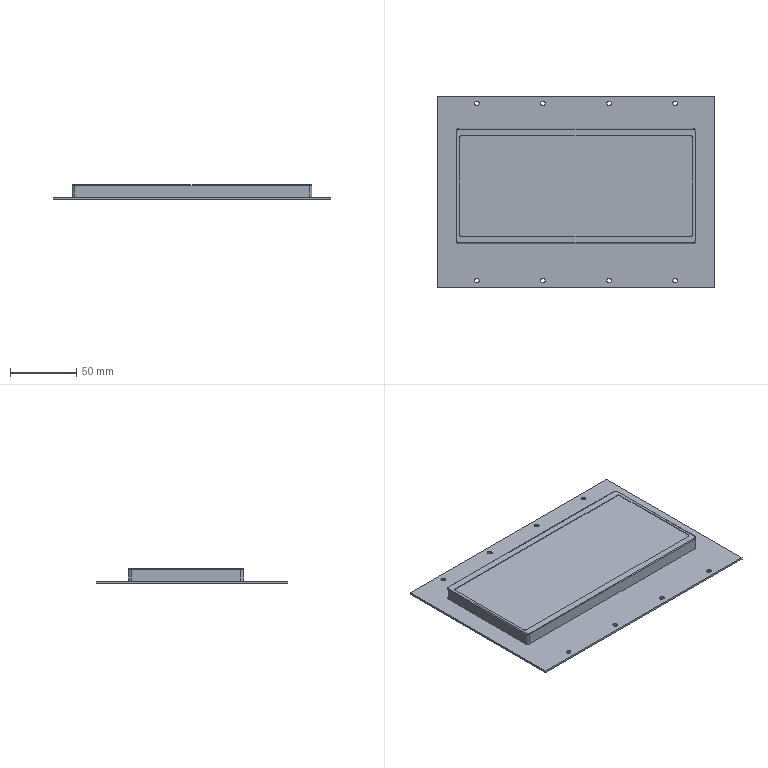Part | STEP file | 1 solid | 40 faces | box 210 x 145 x 11 mm | volume 188408 mm3 | cylinder 20 | plane 16 | torus 4 | commonest cylinder face diameters 3.5 x8 1 x4 3 x4 4 x4